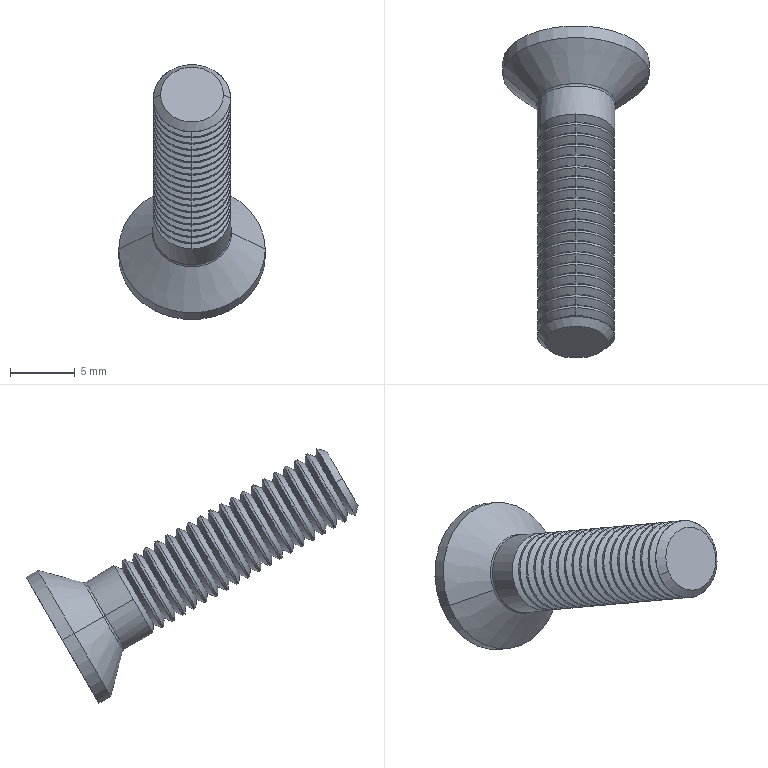Part | STEP file | Socket Countersunk Head Screw_ISO(ISO 10642 - M6 x 25 --- 25S)_Valor predeterminado | 1 solid | 140 faces | box 11.34 x 25.708 x 19.731 mm | volume 759.97 mm3 | cone 82 | cylinder 42 | plane 14 | torus 2 | commonest cylinder face diameters 6 x40 11.34 x2